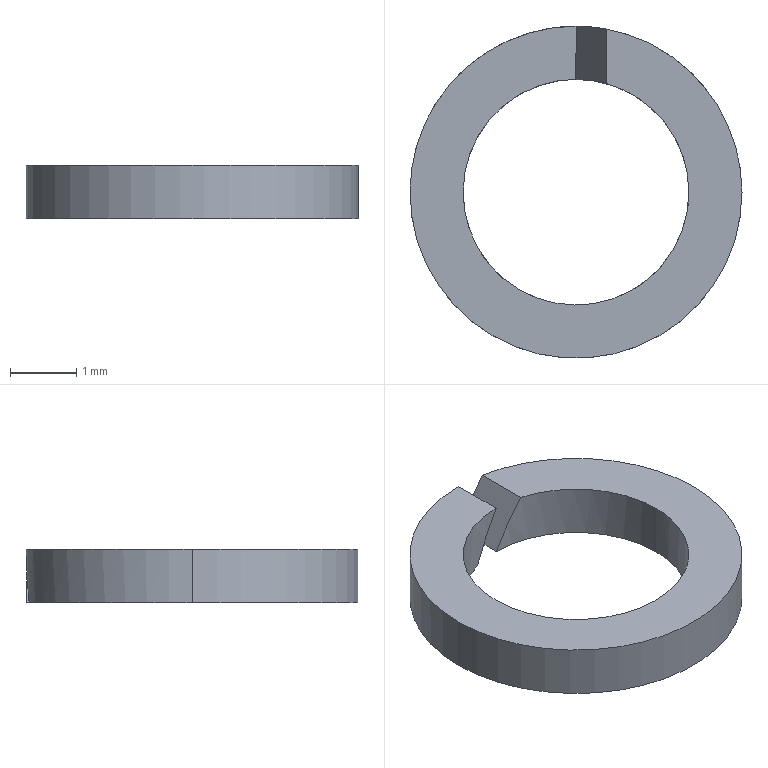Part | STEP file | PN_0015_Default<As Machined> | 1 solid | 10 faces | box 5 x 5 x 0.8 mm | volume 8.148 mm3 | cylinder 6 | plane 4 | commonest cylinder face diameters 3.4 x3 5 x3
STEP:
#1=CARTESIAN_POINT('',(-1.7,0.,-0.8));
#2=VERTEX_POINT('',#1);
#3=CARTESIAN_POINT('',(1.7,0.,-0.8));
#4=VERTEX_POINT('',#3);
#5=CARTESIAN_POINT('',(0.,0.,-0.8));
#6=DIRECTION('',(0.,0.,1.));
#7=AXIS2_PLACEMENT_3D('',#5,#6,$);
#8=CIRCLE('',#7,1.7);
#9=EDGE_CURVE('',#2,#4,#8,.T.);
#10=ORIENTED_EDGE('',*,*,#9,.F.);
#11=CARTESIAN_POINT('',(-1.7,0.,0.));
#12=VERTEX_POINT('',#11);
#13=CARTESIAN_POINT('',(-1.7,0.,-0.8));
#14=DIRECTION('',(0.,0.,1.));
#15=VECTOR('',#14,1.);
#16=LINE('',#13,#15);
#17=EDGE_CURVE('',#2,#12,#16,.T.);
#18=ORIENTED_EDGE('',*,*,#17,.T.);
#19=CARTESIAN_POINT('',(1.7,0.,0.000000001));
#20=VERTEX_POINT('',#19);
#21=CARTESIAN_POINT('',(-1.7,0.,0.));
#22=CARTESIAN_POINT('',(-1.7,-0.5341,0.));
#23=CARTESIAN_POINT('',(-1.49,-1.068,0.));
#24=CARTESIAN_POINT('',(-1.068,-1.49,0.));
#25=CARTESIAN_POINT('',(0.,-1.91,0.));
#26=CARTESIAN_POINT('',(1.068,-1.49,0.000000001));
#27=CARTESIAN_POINT('',(1.49,-1.068,0.000000001));
#28=CARTESIAN_POINT('',(1.7,-0.5341,0.000000001));
#29=CARTESIAN_POINT('',(1.7,0.,0.000000001));
#30=B_SPLINE_CURVE_WITH_KNOTS('',5,(#21,#22,#23,#24,#25,#26,#27,#28,#29),.UNSPECIFIED.,.F.,.U.,(6,3,6),(-2.67,0.,2.67),.UNSPECIFIED.);
#31=EDGE_CURVE('',#12,#20,#30,.T.);
#32=ORIENTED_EDGE('',*,*,#31,.T.);
#33=CARTESIAN_POINT('',(1.7,0.,-0.8));
#34=DIRECTION('',(0.,0.,1.));
#35=VECTOR('',#34,1.);
#36=LINE('',#33,#35);
#37=EDGE_CURVE('',#4,#20,#36,.T.);
#38=ORIENTED_EDGE('',*,*,#37,.F.);
#39=EDGE_LOOP('',(#10,#18,#32,#38));
#40=FACE_OUTER_BOUND('',#39,.T.);
#41=CARTESIAN_POINT('',(0.,0.,-0.8));
#42=DIRECTION('',(0.,0.,1.));
#43=DIRECTION('',(-1.,0.,0.));
#44=AXIS2_PLACEMENT_3D('',#41,#42,#43);
#45=CYLINDRICAL_SURFACE('',#44,1.7);
#46=ADVANCED_FACE('',(#40),#45,.F.);
#47=CARTESIAN_POINT('',(-0.4619,2.457,-0.8));
#48=VERTEX_POINT('',#47);
#49=CARTESIAN_POINT('',(-0.4619,1.636,-0.8));
#50=VERTEX_POINT('',#49);
#51=CARTESIAN_POINT('',(-0.4619,2.047,-0.8));
#52=DIRECTION('',(0.,-1.,0.));
#53=VECTOR('',#52,1.);
#54=LINE('',#51,#53);
#55=EDGE_CURVE('',#48,#50,#54,.T.);
#56=ORIENTED_EDGE('',*,*,#55,.T.);
#57=CARTESIAN_POINT('',(0.,0.000000002,-0.8));
#58=DIRECTION('',(0.,0.,1.));
#59=AXIS2_PLACEMENT_3D('',#57,#58,$);
#60=CIRCLE('',#59,1.7);
#61=EDGE_CURVE('',#50,#2,#60,.T.);
#62=ORIENTED_EDGE('',*,*,#61,.T.);
#63=ORIENTED_EDGE('',*,*,#9,.T.);
#64=CARTESIAN_POINT('',(0.,1.7,-0.8));
#65=VERTEX_POINT('',#64);
#66=CARTESIAN_POINT('',(0.,0.,-0.8));
#67=DIRECTION('',(0.,0.,1.));
#68=AXIS2_PLACEMENT_3D('',#66,#67,$);
#69=CIRCLE('',#68,1.7);
#70=EDGE_CURVE('',#4,#65,#69,.T.);
#71=ORIENTED_EDGE('',*,*,#70,.T.);
#72=CARTESIAN_POINT('',(0.,2.5,-0.8));
#73=VERTEX_POINT('',#72);
#74=CARTESIAN_POINT('',(0.,2.1,-0.8));
#75=DIRECTION('',(0.,-1.,0.));
#76=VECTOR('',#75,1.);
#77=LINE('',#74,#76);
#78=EDGE_CURVE('',#73,#65,#77,.T.);
#79=ORIENTED_EDGE('',*,*,#78,.F.);
#80=CARTESIAN_POINT('',(2.5,0.,-0.8));
#81=VERTEX_POINT('',#80);
#82=CARTESIAN_POINT('',(-0.000000002,-0.000000002,-0.8));
#83=DIRECTION('',(0.,0.,1.));
#84=AXIS2_PLACEMENT_3D('',#82,#83,$);
#85=CIRCLE('',#84,2.5);
#86=EDGE_CURVE('',#81,#73,#85,.T.);
#87=ORIENTED_EDGE('',*,*,#86,.F.);
#88=CARTESIAN_POINT('',(-2.5,0.,-0.8));
#89=VERTEX_POINT('',#88);
#90=CARTESIAN_POINT('',(0.,0.,-0.8));
#91=DIRECTION('',(0.,0.,1.));
#92=AXIS2_PLACEMENT_3D('',#90,#91,$);
#93=CIRCLE('',#92,2.5);
#94=EDGE_CURVE('',#89,#81,#93,.T.);
#95=ORIENTED_EDGE('',*,*,#94,.F.);
#96=CARTESIAN_POINT('',(0.,0.,-0.8));
#97=DIRECTION('',(0.,0.,1.));
#98=AXIS2_PLACEMENT_3D('',#96,#97,$);
#99=CIRCLE('',#98,2.5);
#100=EDGE_CURVE('',#48,#89,#99,.T.);
#101=ORIENTED_EDGE('',*,*,#100,.F.);
#102=EDGE_LOOP('',(#56,#62,#63,#71,#79,#87,#95,#101));
#103=FACE_OUTER_BOUND('',#102,.T.);
#104=CARTESIAN_POINT('',(0.,0.,-0.8));
#105=DIRECTION('',(0.,0.,1.));
#106=DIRECTION('',(1.,0.,0.));
#107=AXIS2_PLACEMENT_3D('',#104,#105,#106);
#108=PLANE('',#107);
#109=ADVANCED_FACE('',(#103),#108,.F.);
#110=ORIENTED_EDGE('',*,*,#17,.F.);
#111=ORIENTED_EDGE('',*,*,#61,.F.);
#112=CARTESIAN_POINT('',(0.,1.7,0.));
#113=VERTEX_POINT('',#112);
#114=CARTESIAN_POINT('',(0.,1.7,0.000000001));
#115=CARTESIAN_POINT('',(-0.1549,1.7,-0.2684));
#116=CARTESIAN_POINT('',(-0.3107,1.679,-0.5381));
#117=CARTESIAN_POINT('',(-0.4619,1.636,-0.8));
#118=B_SPLINE_CURVE_WITH_KNOTS('',3,(#114,#115,#116,#117),.UNSPECIFIED.,.F.,.U.,(4,4),(0.,1.311),.UNSPECIFIED.);
#119=EDGE_CURVE('',#113,#50,#118,.T.);
#120=ORIENTED_EDGE('',*,*,#119,.F.);
#121=CARTESIAN_POINT('',(0.,0.,0.000000001));
#122=DIRECTION('',(0.,0.,1.));
#123=AXIS2_PLACEMENT_3D('',#121,#122,$);
#124=CIRCLE('',#123,1.7);
#125=EDGE_CURVE('',#113,#12,#124,.T.);
#126=ORIENTED_EDGE('',*,*,#125,.T.);
#127=EDGE_LOOP('',(#110,#111,#120,#126));
#128=FACE_OUTER_BOUND('',#127,.T.);
#129=CARTESIAN_POINT('',(0.,0.,-0.8));
#130=DIRECTION('',(0.,0.,1.));
#131=DIRECTION('',(1.,0.,0.));
#132=AXIS2_PLACEMENT_3D('',#129,#130,#131);
#133=CYLINDRICAL_SURFACE('',#132,1.7);
#134=ADVANCED_FACE('',(#128),#133,.F.);
#135=ORIENTED_EDGE('',*,*,#125,.F.);
#136=CARTESIAN_POINT('',(0.,2.5,0.000000001));
#137=VERTEX_POINT('',#136);
#138=CARTESIAN_POINT('',(0.,2.1,0.));
#139=DIRECTION('',(0.,-1.,0.));
#140=VECTOR('',#139,1.);
#141=LINE('',#138,#140);
#142=EDGE_CURVE('',#137,#113,#141,.T.);
#143=ORIENTED_EDGE('',*,*,#142,.F.);
#144=CARTESIAN_POINT('',(-2.5,0.,0.000000001));
#145=VERTEX_POINT('',#144);
#146=CARTESIAN_POINT('',(0.000000002,-0.000000002,0.));
#147=DIRECTION('',(0.,0.,1.));
#148=AXIS2_PLACEMENT_3D('',#146,#147,$);
#149=CIRCLE('',#148,2.5);
#150=EDGE_CURVE('',#137,#145,#149,.T.);
#151=ORIENTED_EDGE('',*,*,#150,.T.);
#152=CARTESIAN_POINT('',(2.5,0.,0.000000001));
#153=VERTEX_POINT('',#152);
#154=CARTESIAN_POINT('',(0.,0.,0.));
#155=DIRECTION('',(0.,0.,1.));
#156=AXIS2_PLACEMENT_3D('',#154,#155,$);
#157=CIRCLE('',#156,2.5);
#158=EDGE_CURVE('',#145,#153,#157,.T.);
#159=ORIENTED_EDGE('',*,*,#158,.T.);
#160=CARTESIAN_POINT('',(0.4619,2.457,0.000000001));
#161=VERTEX_POINT('',#160);
#162=CARTESIAN_POINT('',(0.,0.,0.));
#163=DIRECTION('',(0.,0.,1.));
#164=AXIS2_PLACEMENT_3D('',#162,#163,$);
#165=CIRCLE('',#164,2.5);
#166=EDGE_CURVE('',#153,#161,#165,.T.);
#167=ORIENTED_EDGE('',*,*,#166,.T.);
#168=CARTESIAN_POINT('',(0.4619,1.636,0.000000001));
#169=VERTEX_POINT('',#168);
#170=CARTESIAN_POINT('',(0.4619,2.047,0.));
#171=DIRECTION('',(0.,-1.,0.));
#172=VECTOR('',#171,1.);
#173=LINE('',#170,#172);
#174=EDGE_CURVE('',#161,#169,#173,.T.);
#175=ORIENTED_EDGE('',*,*,#174,.T.);
#176=CARTESIAN_POINT('',(0.,0.000000002,0.));
#177=DIRECTION('',(0.,0.,1.));
#178=AXIS2_PLACEMENT_3D('',#176,#177,$);
#179=CIRCLE('',#178,1.7);
#180=EDGE_CURVE('',#20,#169,#179,.T.);
#181=ORIENTED_EDGE('',*,*,#180,.F.);
#182=ORIENTED_EDGE('',*,*,#31,.F.);
#183=EDGE_LOOP('',(#135,#143,#151,#159,#167,#175,#181,#182));
#184=FACE_OUTER_BOUND('',#183,.T.);
#185=CARTESIAN_POINT('',(0.,0.,0.));
#186=DIRECTION('',(0.,0.,1.));
#187=DIRECTION('',(1.,0.,0.));
#188=AXIS2_PLACEMENT_3D('',#185,#186,#187);
#189=PLANE('',#188);
#190=ADVANCED_FACE('',(#184),#189,.T.);
#191=ORIENTED_EDGE('',*,*,#70,.F.);
#192=ORIENTED_EDGE('',*,*,#37,.T.);
#193=ORIENTED_EDGE('',*,*,#180,.T.);
#194=CARTESIAN_POINT('',(0.,1.7,-0.8));
#195=CARTESIAN_POINT('',(0.1549,1.7,-0.5316));
#196=CARTESIAN_POINT('',(0.3107,1.679,-0.2619));
#197=CARTESIAN_POINT('',(0.4619,1.636,0.000000001));
#198=B_SPLINE_CURVE_WITH_KNOTS('',3,(#194,#195,#196,#197),.UNSPECIFIED.,.F.,.U.,(4,4),(0.,1.311),.UNSPECIFIED.);
#199=EDGE_CURVE('',#65,#169,#198,.T.);
#200=ORIENTED_EDGE('',*,*,#199,.F.);
#201=EDGE_LOOP('',(#191,#192,#193,#200));
#202=FACE_OUTER_BOUND('',#201,.T.);
#203=CARTESIAN_POINT('',(0.,0.,-0.8));
#204=DIRECTION('',(0.,0.,1.));
#205=DIRECTION('',(1.,0.,0.));
#206=AXIS2_PLACEMENT_3D('',#203,#204,#205);
#207=CYLINDRICAL_SURFACE('',#206,1.7);
#208=ADVANCED_FACE('',(#202),#207,.F.);
#209=ORIENTED_EDGE('',*,*,#142,.T.);
#210=ORIENTED_EDGE('',*,*,#119,.T.);
#211=ORIENTED_EDGE('',*,*,#55,.F.);
#212=CARTESIAN_POINT('',(0.,2.5,0.));
#213=CARTESIAN_POINT('',(-0.09263,2.5,-0.1604));
#214=CARTESIAN_POINT('',(-0.1854,2.496,-0.321));
#215=CARTESIAN_POINT('',(-0.278,2.487,-0.4816));
#216=CARTESIAN_POINT('',(-0.3703,2.474,-0.6413));
#217=CARTESIAN_POINT('',(-0.4619,2.457,-0.8));
#218=B_SPLINE_CURVE_WITH_KNOTS('',5,(#212,#213,#214,#215,#216,#217),.UNSPECIFIED.,.F.,.U.,(6,6),(0.,1.308),.UNSPECIFIED.);
#219=EDGE_CURVE('',#137,#48,#218,.T.);
#220=ORIENTED_EDGE('',*,*,#219,.F.);
#221=EDGE_LOOP('',(#209,#210,#211,#220));
#222=FACE_OUTER_BOUND('',#221,.T.);
#223=CARTESIAN_POINT('',(0.,2.5,0.));
#224=DIRECTION('',(0.866,0.,-0.5));
#225=DIRECTION('',(-0.5,0.,-0.866));
#226=AXIS2_PLACEMENT_3D('',#223,#224,#225);
#227=PLANE('',#226);
#228=ADVANCED_FACE('',(#222),#227,.T.);
#229=ORIENTED_EDGE('',*,*,#78,.T.);
#230=ORIENTED_EDGE('',*,*,#199,.T.);
#231=ORIENTED_EDGE('',*,*,#174,.F.);
#232=CARTESIAN_POINT('',(0.,2.5,-0.8));
#233=CARTESIAN_POINT('',(0.09263,2.5,-0.6396));
#234=CARTESIAN_POINT('',(0.1854,2.496,-0.479));
#235=CARTESIAN_POINT('',(0.278,2.487,-0.3184));
#236=CARTESIAN_POINT('',(0.3703,2.474,-0.1587));
#237=CARTESIAN_POINT('',(0.4619,2.457,0.));
#238=B_SPLINE_CURVE_WITH_KNOTS('',5,(#232,#233,#234,#235,#236,#237),.UNSPECIFIED.,.F.,.U.,(6,6),(0.,1.308),.UNSPECIFIED.);
#239=EDGE_CURVE('',#73,#161,#238,.T.);
#240=ORIENTED_EDGE('',*,*,#239,.F.);
#241=EDGE_LOOP('',(#229,#230,#231,#240));
#242=FACE_OUTER_BOUND('',#241,.T.);
#243=CARTESIAN_POINT('',(0.,2.5,-0.8));
#244=DIRECTION('',(-0.866,0.,0.5));
#245=DIRECTION('',(0.5,0.,0.866));
#246=AXIS2_PLACEMENT_3D('',#243,#244,#245);
#247=PLANE('',#246);
#248=ADVANCED_FACE('',(#242),#247,.T.);
#249=CARTESIAN_POINT('',(2.5,0.,-0.8));
#250=DIRECTION('',(0.,0.,1.));
#251=VECTOR('',#250,1.);
#252=LINE('',#249,#251);
#253=EDGE_CURVE('',#81,#153,#252,.T.);
#254=ORIENTED_EDGE('',*,*,#253,.F.);
#255=ORIENTED_EDGE('',*,*,#86,.T.);
#256=ORIENTED_EDGE('',*,*,#239,.T.);
#257=ORIENTED_EDGE('',*,*,#166,.F.);
#258=EDGE_LOOP('',(#254,#255,#256,#257));
#259=FACE_OUTER_BOUND('',#258,.T.);
#260=CARTESIAN_POINT('',(0.,0.,-0.8));
#261=DIRECTION('',(0.,0.,1.));
#262=DIRECTION('',(1.,0.,0.));
#263=AXIS2_PLACEMENT_3D('',#260,#261,#262);
#264=CYLINDRICAL_SURFACE('',#263,2.5);
#265=ADVANCED_FACE('',(#259),#264,.T.);
#266=CARTESIAN_POINT('',(-2.5,0.,-0.8));
#267=DIRECTION('',(0.,0.,1.));
#268=VECTOR('',#267,1.);
#269=LINE('',#266,#268);
#270=EDGE_CURVE('',#89,#145,#269,.T.);
#271=ORIENTED_EDGE('',*,*,#270,.F.);
#272=ORIENTED_EDGE('',*,*,#94,.T.);
#273=ORIENTED_EDGE('',*,*,#253,.T.);
#274=ORIENTED_EDGE('',*,*,#158,.F.);
#275=EDGE_LOOP('',(#271,#272,#273,#274));
#276=FACE_OUTER_BOUND('',#275,.T.);
#277=CARTESIAN_POINT('',(0.,0.,-0.8));
#278=DIRECTION('',(0.,0.,1.));
#279=DIRECTION('',(-1.,0.,0.));
#280=AXIS2_PLACEMENT_3D('',#277,#278,#279);
#281=CYLINDRICAL_SURFACE('',#280,2.5);
#282=ADVANCED_FACE('',(#276),#281,.T.);
#283=ORIENTED_EDGE('',*,*,#100,.T.);
#284=ORIENTED_EDGE('',*,*,#270,.T.);
#285=ORIENTED_EDGE('',*,*,#150,.F.);
#286=ORIENTED_EDGE('',*,*,#219,.T.);
#287=EDGE_LOOP('',(#283,#284,#285,#286));
#288=FACE_OUTER_BOUND('',#287,.T.);
#289=CARTESIAN_POINT('',(0.,0.,-0.8));
#290=DIRECTION('',(0.,0.,1.));
#291=DIRECTION('',(1.,0.,0.));
#292=AXIS2_PLACEMENT_3D('',#289,#290,#291);
#293=CYLINDRICAL_SURFACE('',#292,2.5);
#294=ADVANCED_FACE('',(#288),#293,.T.);
#295=CLOSED_SHELL('',(#46,#109,#134,#190,#208,#228,#248,#265,#282,#294));
#296=MANIFOLD_SOLID_BREP('',#295);
#297=(LENGTH_UNIT()NAMED_UNIT(*)SI_UNIT(.MILLI.,.METRE.));
#298=UNCERTAINTY_MEASURE_WITH_UNIT(LENGTH_MEASURE(0.005),#297,'','');
#299=(NAMED_UNIT(*)PLANE_ANGLE_UNIT()SI_UNIT($,.RADIAN.));
#300=(NAMED_UNIT(*)SI_UNIT($,.STERADIAN.)SOLID_ANGLE_UNIT());
#301=(GEOMETRIC_REPRESENTATION_CONTEXT(3)GLOBAL_UNCERTAINTY_ASSIGNED_CONTEXT((#298))GLOBAL_UNIT_ASSIGNED_CONTEXT((#297,#299,#300))REPRESENTATION_CONTEXT('',''));
#302=ADVANCED_BREP_SHAPE_REPRESENTATION('',(#296),#301);